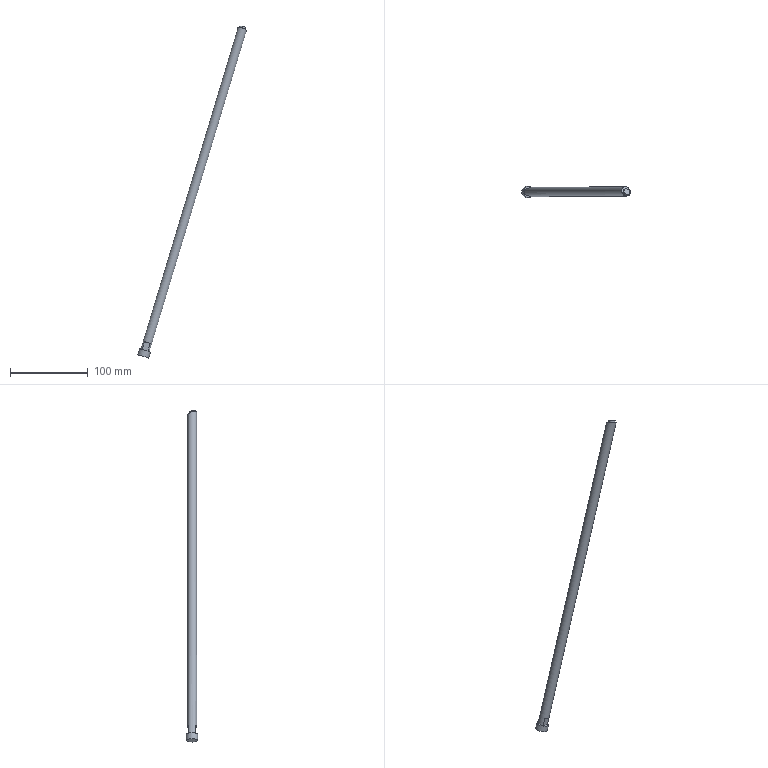Part | STEP file | solid 97 | 1 solid | 12 faces | box 140.241 x 15 x 428.298 mm | volume 50261 mm3 | plane 8 | cylinder 3 | other 1 | commonest cylinder face diameters 8.04 x1 12 x1 15 x1